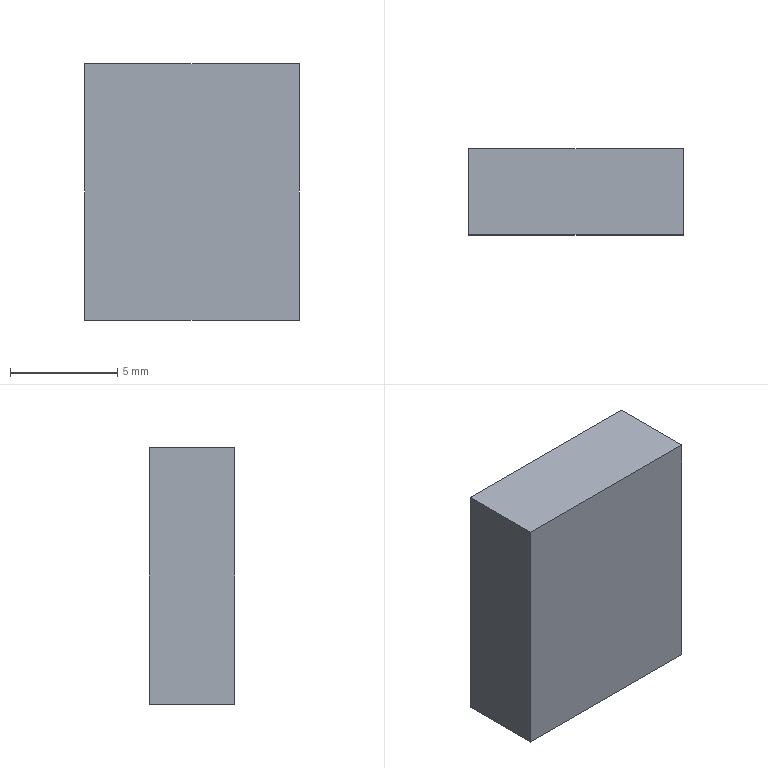Part | STEP file | X77b-01016 | 1 solid | 6 faces | box 10 x 4 x 12 mm | volume 480 mm3 | plane 6
STEP:
#1=CARTESIAN_POINT('',(-34.489,-84.175,0.));
#2=VERTEX_POINT('',#1);
#3=CARTESIAN_POINT('',(-34.489,-88.175,0.));
#4=VERTEX_POINT('',#3);
#5=CARTESIAN_POINT('',(-34.489,-84.175,0.));
#6=DIRECTION('',(0.,-1.,0.));
#7=VECTOR('',#6,1000.);
#8=LINE('',#5,#7);
#9=EDGE_CURVE('',#2,#4,#8,.T.);
#10=ORIENTED_EDGE('',*,*,#9,.F.);
#11=CARTESIAN_POINT('',(-34.489,-84.175,-12.));
#12=VERTEX_POINT('',#11);
#13=CARTESIAN_POINT('',(-34.489,-84.175,-12.));
#14=DIRECTION('',(0.,0.,1.));
#15=VECTOR('',#14,1000.);
#16=LINE('',#13,#15);
#17=EDGE_CURVE('',#12,#2,#16,.T.);
#18=ORIENTED_EDGE('',*,*,#17,.F.);
#19=CARTESIAN_POINT('',(-34.489,-88.175,-12.));
#20=VERTEX_POINT('',#19);
#21=CARTESIAN_POINT('',(-34.489,-84.175,-12.));
#22=DIRECTION('',(0.,-1.,0.));
#23=VECTOR('',#22,1000.);
#24=LINE('',#21,#23);
#25=EDGE_CURVE('',#12,#20,#24,.T.);
#26=ORIENTED_EDGE('',*,*,#25,.T.);
#27=CARTESIAN_POINT('',(-34.489,-88.175,-12.));
#28=DIRECTION('',(0.,0.,1.));
#29=VECTOR('',#28,1000.);
#30=LINE('',#27,#29);
#31=EDGE_CURVE('',#20,#4,#30,.T.);
#32=ORIENTED_EDGE('',*,*,#31,.T.);
#33=EDGE_LOOP('',(#10,#18,#26,#32));
#34=FACE_OUTER_BOUND('',#33,.T.);
#35=CARTESIAN_POINT('',(-34.489,-84.175,-12.));
#36=DIRECTION('',(-1.,0.,0.));
#37=DIRECTION('',(0.,0.,1.));
#38=AXIS2_PLACEMENT_3D('',#35,#36,#37);
#39=PLANE('',#38);
#40=ADVANCED_FACE('',(#34),#39,.T.);
#41=CARTESIAN_POINT('',(-24.489,-84.175,0.));
#42=VERTEX_POINT('',#41);
#43=CARTESIAN_POINT('',(-34.489,-84.175,0.));
#44=DIRECTION('',(-1.,0.,0.));
#45=VECTOR('',#44,1000.);
#46=LINE('',#43,#45);
#47=EDGE_CURVE('',#42,#2,#46,.T.);
#48=ORIENTED_EDGE('',*,*,#47,.F.);
#49=CARTESIAN_POINT('',(-24.489,-84.175,-12.));
#50=VERTEX_POINT('',#49);
#51=CARTESIAN_POINT('',(-24.489,-84.175,-12.));
#52=DIRECTION('',(0.,0.,1.));
#53=VECTOR('',#52,1000.);
#54=LINE('',#51,#53);
#55=EDGE_CURVE('',#50,#42,#54,.T.);
#56=ORIENTED_EDGE('',*,*,#55,.F.);
#57=CARTESIAN_POINT('',(-34.489,-84.175,-12.));
#58=DIRECTION('',(-1.,0.,0.));
#59=VECTOR('',#58,1000.);
#60=LINE('',#57,#59);
#61=EDGE_CURVE('',#50,#12,#60,.T.);
#62=ORIENTED_EDGE('',*,*,#61,.T.);
#63=ORIENTED_EDGE('',*,*,#17,.T.);
#64=EDGE_LOOP('',(#48,#56,#62,#63));
#65=FACE_OUTER_BOUND('',#64,.T.);
#66=CARTESIAN_POINT('',(-34.489,-84.175,-12.));
#67=DIRECTION('',(0.,1.,0.));
#68=DIRECTION('',(0.,0.,1.));
#69=AXIS2_PLACEMENT_3D('',#66,#67,#68);
#70=PLANE('',#69);
#71=ADVANCED_FACE('',(#65),#70,.T.);
#72=CARTESIAN_POINT('',(-24.489,-88.175,0.));
#73=VERTEX_POINT('',#72);
#74=CARTESIAN_POINT('',(-24.489,-84.175,0.));
#75=DIRECTION('',(0.,1.,0.));
#76=VECTOR('',#75,1000.);
#77=LINE('',#74,#76);
#78=EDGE_CURVE('',#73,#42,#77,.T.);
#79=ORIENTED_EDGE('',*,*,#78,.F.);
#80=CARTESIAN_POINT('',(-24.489,-88.175,-12.));
#81=VERTEX_POINT('',#80);
#82=CARTESIAN_POINT('',(-24.489,-88.175,-12.));
#83=DIRECTION('',(0.,0.,1.));
#84=VECTOR('',#83,1000.);
#85=LINE('',#82,#84);
#86=EDGE_CURVE('',#81,#73,#85,.T.);
#87=ORIENTED_EDGE('',*,*,#86,.F.);
#88=CARTESIAN_POINT('',(-24.489,-84.175,-12.));
#89=DIRECTION('',(0.,1.,0.));
#90=VECTOR('',#89,1000.);
#91=LINE('',#88,#90);
#92=EDGE_CURVE('',#81,#50,#91,.T.);
#93=ORIENTED_EDGE('',*,*,#92,.T.);
#94=ORIENTED_EDGE('',*,*,#55,.T.);
#95=EDGE_LOOP('',(#79,#87,#93,#94));
#96=FACE_OUTER_BOUND('',#95,.T.);
#97=CARTESIAN_POINT('',(-24.489,-84.175,-12.));
#98=DIRECTION('',(1.,0.,0.));
#99=DIRECTION('',(0.,0.,-1.));
#100=AXIS2_PLACEMENT_3D('',#97,#98,#99);
#101=PLANE('',#100);
#102=ADVANCED_FACE('',(#96),#101,.T.);
#103=CARTESIAN_POINT('',(-34.489,-88.175,0.));
#104=DIRECTION('',(1.,0.,0.));
#105=VECTOR('',#104,1000.);
#106=LINE('',#103,#105);
#107=EDGE_CURVE('',#4,#73,#106,.T.);
#108=ORIENTED_EDGE('',*,*,#107,.F.);
#109=ORIENTED_EDGE('',*,*,#31,.F.);
#110=CARTESIAN_POINT('',(-34.489,-88.175,-12.));
#111=DIRECTION('',(1.,0.,0.));
#112=VECTOR('',#111,1000.);
#113=LINE('',#110,#112);
#114=EDGE_CURVE('',#20,#81,#113,.T.);
#115=ORIENTED_EDGE('',*,*,#114,.T.);
#116=ORIENTED_EDGE('',*,*,#86,.T.);
#117=EDGE_LOOP('',(#108,#109,#115,#116));
#118=FACE_OUTER_BOUND('',#117,.T.);
#119=CARTESIAN_POINT('',(-34.489,-88.175,-12.));
#120=DIRECTION('',(0.,-1.,0.));
#121=DIRECTION('',(0.,0.,-1.));
#122=AXIS2_PLACEMENT_3D('',#119,#120,#121);
#123=PLANE('',#122);
#124=ADVANCED_FACE('',(#118),#123,.T.);
#125=ORIENTED_EDGE('',*,*,#25,.F.);
#126=ORIENTED_EDGE('',*,*,#61,.F.);
#127=ORIENTED_EDGE('',*,*,#92,.F.);
#128=ORIENTED_EDGE('',*,*,#114,.F.);
#129=EDGE_LOOP('',(#125,#126,#127,#128));
#130=FACE_OUTER_BOUND('',#129,.T.);
#131=CARTESIAN_POINT('',(-34.489,-88.175,-12.));
#132=DIRECTION('',(0.,0.,1.));
#133=DIRECTION('',(1.,0.,0.));
#134=AXIS2_PLACEMENT_3D('',#131,#132,#133);
#135=PLANE('',#134);
#136=ADVANCED_FACE('',(#130),#135,.F.);
#137=ORIENTED_EDGE('',*,*,#9,.T.);
#138=ORIENTED_EDGE('',*,*,#107,.T.);
#139=ORIENTED_EDGE('',*,*,#78,.T.);
#140=ORIENTED_EDGE('',*,*,#47,.T.);
#141=EDGE_LOOP('',(#137,#138,#139,#140));
#142=FACE_OUTER_BOUND('',#141,.T.);
#143=CARTESIAN_POINT('',(-34.489,-88.175,0.));
#144=DIRECTION('',(0.,0.,1.));
#145=DIRECTION('',(1.,0.,0.));
#146=AXIS2_PLACEMENT_3D('',#143,#144,#145);
#147=PLANE('',#146);
#148=ADVANCED_FACE('',(#142),#147,.T.);
#149=CLOSED_SHELL('',(#40,#71,#102,#124,#136,#148));
#150=MANIFOLD_SOLID_BREP('',#149);
#151=CARTESIAN_POINT('',(0.,0.,0.));
#152=DIRECTION('',(0.,0.,1.));
#153=DIRECTION('',(1.,0.,0.));
#154=AXIS2_PLACEMENT_3D('',#151,#152,#153);
#155=(LENGTH_UNIT()NAMED_UNIT(*)SI_UNIT(.MILLI.,.METRE.));
#156=UNCERTAINTY_MEASURE_WITH_UNIT(LENGTH_MEASURE(0.00001),#155,'','');
#157=(NAMED_UNIT(*)PLANE_ANGLE_UNIT()SI_UNIT($,.RADIAN.));
#158=(NAMED_UNIT(*)SI_UNIT($,.STERADIAN.)SOLID_ANGLE_UNIT());
#159=(GEOMETRIC_REPRESENTATION_CONTEXT(3)GLOBAL_UNCERTAINTY_ASSIGNED_CONTEXT((#156))GLOBAL_UNIT_ASSIGNED_CONTEXT((#155,#157,#158))REPRESENTATION_CONTEXT('',''));
#160=ADVANCED_BREP_SHAPE_REPRESENTATION('',(#150,#154),#159);